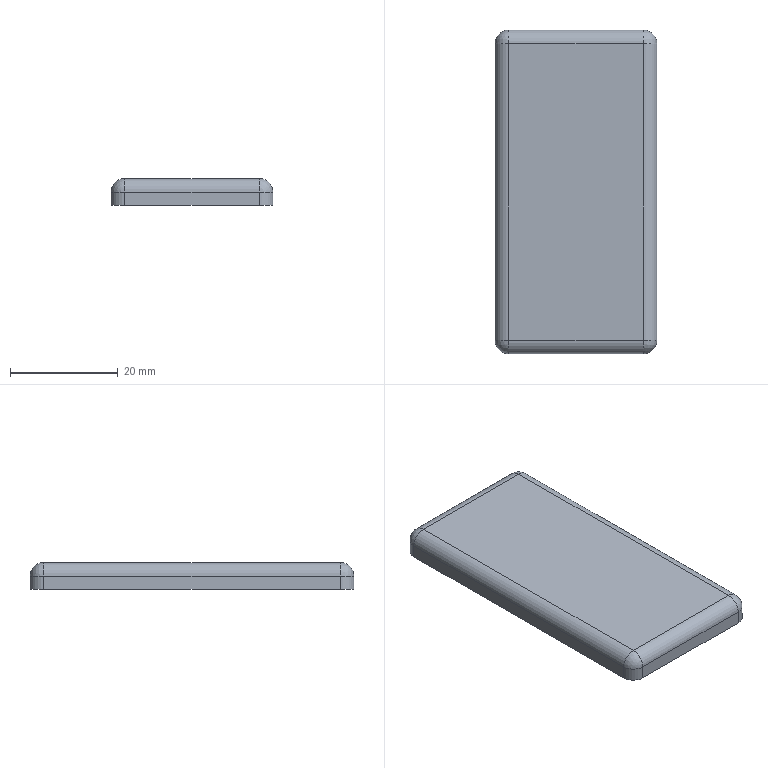Part | STEP file | Aluminium profile end cover plate | 1 solid | 18 faces | box 30 x 60 x 5 mm | volume 8742 mm3 | cylinder 8 | plane 6 | sphere 4 | commonest cylinder face diameters 5 x8
STEP:
#1=CARTESIAN_POINT('',(0.,0.,0.));
#2=DIRECTION('',(0.,0.,1.));
#3=DIRECTION('',(1.,0.,0.));
#4=AXIS2_PLACEMENT_3D('',#1,#2,#3);
#5=CARTESIAN_POINT('',(15.,27.5,2.5));
#6=VERTEX_POINT('',#5);
#7=CARTESIAN_POINT('',(15.,-27.5,2.5));
#8=VERTEX_POINT('',#7);
#9=CARTESIAN_POINT('',(15.,-30.,2.5));
#10=DIRECTION('',(0.,-1.,0.));
#11=VECTOR('',#10,1.);
#12=LINE('',#9,#11);
#13=CARTESIAN_POINT('',(15.,30.,5.));
#14=DIRECTION('',(-1.,0.,0.));
#15=DIRECTION('',(0.,-1.,0.));
#16=AXIS2_PLACEMENT_3D('',#13,#14,#15);
#17=PLANE('',#16);
#18=CARTESIAN_POINT('',(60.,-2.5));
#19=DIRECTION('',(1.,0.));
#20=VECTOR('',#19,1.);
#21=LINE('',#18,#20);
#22=(GEOMETRIC_REPRESENTATION_CONTEXT(2)PARAMETRIC_REPRESENTATION_CONTEXT()REPRESENTATION_CONTEXT('',''));
#23=DEFINITIONAL_REPRESENTATION('',(#21),#22);
#24=PCURVE('',#17,#23);
#25=CARTESIAN_POINT('',(12.5,0.,2.5));
#26=DIRECTION('',(0.,-1.,0.));
#27=DIRECTION('',(1.,0.,0.));
#28=AXIS2_PLACEMENT_3D('',#25,#26,#27);
#29=CYLINDRICAL_SURFACE('',#28,2.5);
#30=CARTESIAN_POINT('',(0.,30.));
#31=DIRECTION('',(0.,1.));
#32=VECTOR('',#31,1.);
#33=LINE('',#30,#32);
#34=(GEOMETRIC_REPRESENTATION_CONTEXT(2)PARAMETRIC_REPRESENTATION_CONTEXT()REPRESENTATION_CONTEXT('',''));
#35=DEFINITIONAL_REPRESENTATION('',(#33),#34);
#36=PCURVE('',#29,#35);
#37=SURFACE_CURVE('',#12,(#24,#36),.PCURVE_S1.);
#38=EDGE_CURVE('',#6,#8,#37,.T.);
#39=ORIENTED_EDGE('',*,*,#38,.T.);
#40=CARTESIAN_POINT('',(15.,-27.5,0.));
#41=VERTEX_POINT('',#40);
#42=CARTESIAN_POINT('',(15.,-27.5,5.));
#43=DIRECTION('',(0.,0.,-1.));
#44=VECTOR('',#43,1.);
#45=LINE('',#42,#44);
#46=CARTESIAN_POINT('',(57.5,0.));
#47=DIRECTION('',(0.,-1.));
#48=VECTOR('',#47,1.);
#49=LINE('',#46,#48);
#50=(GEOMETRIC_REPRESENTATION_CONTEXT(2)PARAMETRIC_REPRESENTATION_CONTEXT()REPRESENTATION_CONTEXT('',''));
#51=DEFINITIONAL_REPRESENTATION('',(#49),#50);
#52=PCURVE('',#17,#51);
#53=CARTESIAN_POINT('',(12.5,-27.5,5.));
#54=DIRECTION('',(0.,0.,-1.));
#55=DIRECTION('',(-1.,0.,0.));
#56=AXIS2_PLACEMENT_3D('',#53,#54,#55);
#57=CYLINDRICAL_SURFACE('',#56,2.5);
#58=CARTESIAN_POINT('',(3.142,0.));
#59=DIRECTION('',(0.,1.));
#60=VECTOR('',#59,1.);
#61=LINE('',#58,#60);
#62=(GEOMETRIC_REPRESENTATION_CONTEXT(2)PARAMETRIC_REPRESENTATION_CONTEXT()REPRESENTATION_CONTEXT('',''));
#63=DEFINITIONAL_REPRESENTATION('',(#61),#62);
#64=PCURVE('',#57,#63);
#65=SURFACE_CURVE('',#45,(#52,#64),.PCURVE_S1.);
#66=EDGE_CURVE('',#8,#41,#65,.T.);
#67=ORIENTED_EDGE('',*,*,#66,.T.);
#68=CARTESIAN_POINT('',(15.,27.5,0.));
#69=VERTEX_POINT('',#68);
#70=CARTESIAN_POINT('',(15.,30.,0.));
#71=DIRECTION('',(0.,1.,0.));
#72=VECTOR('',#71,1.);
#73=LINE('',#70,#72);
#74=CARTESIAN_POINT('',(0.,-5.));
#75=DIRECTION('',(-1.,0.));
#76=VECTOR('',#75,1.);
#77=LINE('',#74,#76);
#78=(GEOMETRIC_REPRESENTATION_CONTEXT(2)PARAMETRIC_REPRESENTATION_CONTEXT()REPRESENTATION_CONTEXT('',''));
#79=DEFINITIONAL_REPRESENTATION('',(#77),#78);
#80=PCURVE('',#17,#79);
#81=CARTESIAN_POINT('',(0.,0.,0.));
#82=DIRECTION('',(0.,0.,1.));
#83=DIRECTION('',(1.,0.,0.));
#84=AXIS2_PLACEMENT_3D('',#81,#82,#83);
#85=PLANE('',#84);
#86=CARTESIAN_POINT('',(15.,30.));
#87=DIRECTION('',(0.,1.));
#88=VECTOR('',#87,1.);
#89=LINE('',#86,#88);
#90=(GEOMETRIC_REPRESENTATION_CONTEXT(2)PARAMETRIC_REPRESENTATION_CONTEXT()REPRESENTATION_CONTEXT('',''));
#91=DEFINITIONAL_REPRESENTATION('',(#89),#90);
#92=PCURVE('',#85,#91);
#93=SURFACE_CURVE('',#73,(#80,#92),.PCURVE_S1.);
#94=EDGE_CURVE('',#41,#69,#93,.T.);
#95=ORIENTED_EDGE('',*,*,#94,.T.);
#96=CARTESIAN_POINT('',(15.,27.5,5.));
#97=DIRECTION('',(0.,0.,1.));
#98=VECTOR('',#97,1.);
#99=LINE('',#96,#98);
#100=CARTESIAN_POINT('',(2.5,0.));
#101=DIRECTION('',(0.,1.));
#102=VECTOR('',#101,1.);
#103=LINE('',#100,#102);
#104=(GEOMETRIC_REPRESENTATION_CONTEXT(2)PARAMETRIC_REPRESENTATION_CONTEXT()REPRESENTATION_CONTEXT('',''));
#105=DEFINITIONAL_REPRESENTATION('',(#103),#104);
#106=PCURVE('',#17,#105);
#107=CARTESIAN_POINT('',(12.5,27.5,5.));
#108=DIRECTION('',(0.,0.,-1.));
#109=DIRECTION('',(-1.,0.,0.));
#110=AXIS2_PLACEMENT_3D('',#107,#108,#109);
#111=CYLINDRICAL_SURFACE('',#110,2.5);
#112=CARTESIAN_POINT('',(3.142,0.));
#113=DIRECTION('',(0.,-1.));
#114=VECTOR('',#113,1.);
#115=LINE('',#112,#114);
#116=(GEOMETRIC_REPRESENTATION_CONTEXT(2)PARAMETRIC_REPRESENTATION_CONTEXT()REPRESENTATION_CONTEXT('',''));
#117=DEFINITIONAL_REPRESENTATION('',(#115),#116);
#118=PCURVE('',#111,#117);
#119=SURFACE_CURVE('',#99,(#106,#118),.PCURVE_S1.);
#120=EDGE_CURVE('',#69,#6,#119,.T.);
#121=ORIENTED_EDGE('',*,*,#120,.T.);
#122=EDGE_LOOP('',(#39,#67,#95,#121));
#123=FACE_BOUND('',#122,.T.);
#124=ADVANCED_FACE('',(#123),#17,.F.);
#125=CARTESIAN_POINT('',(12.5,30.,0.));
#126=VERTEX_POINT('',#125);
#127=CARTESIAN_POINT('',(-12.5,30.,0.));
#128=VERTEX_POINT('',#127);
#129=CARTESIAN_POINT('',(-15.,30.,0.));
#130=DIRECTION('',(-1.,0.,0.));
#131=VECTOR('',#130,1.);
#132=LINE('',#129,#131);
#133=CARTESIAN_POINT('',(-15.,30.,5.));
#134=DIRECTION('',(0.,-1.,0.));
#135=DIRECTION('',(0.,0.,-1.));
#136=AXIS2_PLACEMENT_3D('',#133,#134,#135);
#137=PLANE('',#136);
#138=CARTESIAN_POINT('',(5.,0.));
#139=DIRECTION('',(0.,-1.));
#140=VECTOR('',#139,1.);
#141=LINE('',#138,#140);
#142=(GEOMETRIC_REPRESENTATION_CONTEXT(2)PARAMETRIC_REPRESENTATION_CONTEXT()REPRESENTATION_CONTEXT('',''));
#143=DEFINITIONAL_REPRESENTATION('',(#141),#142);
#144=PCURVE('',#137,#143);
#145=CARTESIAN_POINT('',(-15.,30.));
#146=DIRECTION('',(-1.,0.));
#147=VECTOR('',#146,1.);
#148=LINE('',#145,#147);
#149=(GEOMETRIC_REPRESENTATION_CONTEXT(2)PARAMETRIC_REPRESENTATION_CONTEXT()REPRESENTATION_CONTEXT('',''));
#150=DEFINITIONAL_REPRESENTATION('',(#148),#149);
#151=PCURVE('',#85,#150);
#152=SURFACE_CURVE('',#132,(#144,#151),.PCURVE_S1.);
#153=EDGE_CURVE('',#126,#128,#152,.T.);
#154=ORIENTED_EDGE('',*,*,#153,.T.);
#155=CARTESIAN_POINT('',(-12.5,30.,2.5));
#156=VERTEX_POINT('',#155);
#157=CARTESIAN_POINT('',(-12.5,30.,5.));
#158=DIRECTION('',(0.,0.,1.));
#159=VECTOR('',#158,1.);
#160=LINE('',#157,#159);
#161=CARTESIAN_POINT('',(0.,2.5));
#162=DIRECTION('',(-1.,0.));
#163=VECTOR('',#162,1.);
#164=LINE('',#161,#163);
#165=(GEOMETRIC_REPRESENTATION_CONTEXT(2)PARAMETRIC_REPRESENTATION_CONTEXT()REPRESENTATION_CONTEXT('',''));
#166=DEFINITIONAL_REPRESENTATION('',(#164),#165);
#167=PCURVE('',#137,#166);
#168=CARTESIAN_POINT('',(-12.5,27.5,5.));
#169=DIRECTION('',(0.,0.,-1.));
#170=DIRECTION('',(-1.,0.,0.));
#171=AXIS2_PLACEMENT_3D('',#168,#169,#170);
#172=CYLINDRICAL_SURFACE('',#171,2.5);
#173=CARTESIAN_POINT('',(1.571,0.));
#174=DIRECTION('',(0.,-1.));
#175=VECTOR('',#174,1.);
#176=LINE('',#173,#175);
#177=(GEOMETRIC_REPRESENTATION_CONTEXT(2)PARAMETRIC_REPRESENTATION_CONTEXT()REPRESENTATION_CONTEXT('',''));
#178=DEFINITIONAL_REPRESENTATION('',(#176),#177);
#179=PCURVE('',#172,#178);
#180=SURFACE_CURVE('',#160,(#167,#179),.PCURVE_S1.);
#181=EDGE_CURVE('',#128,#156,#180,.T.);
#182=ORIENTED_EDGE('',*,*,#181,.T.);
#183=CARTESIAN_POINT('',(12.5,30.,2.5));
#184=VERTEX_POINT('',#183);
#185=CARTESIAN_POINT('',(15.,30.,2.5));
#186=DIRECTION('',(1.,0.,0.));
#187=VECTOR('',#186,1.);
#188=LINE('',#185,#187);
#189=CARTESIAN_POINT('',(2.5,30.));
#190=DIRECTION('',(0.,1.));
#191=VECTOR('',#190,1.);
#192=LINE('',#189,#191);
#193=(GEOMETRIC_REPRESENTATION_CONTEXT(2)PARAMETRIC_REPRESENTATION_CONTEXT()REPRESENTATION_CONTEXT('',''));
#194=DEFINITIONAL_REPRESENTATION('',(#192),#193);
#195=PCURVE('',#137,#194);
#196=CARTESIAN_POINT('',(0.,27.5,2.5));
#197=DIRECTION('',(1.,0.,0.));
#198=DIRECTION('',(0.,0.,-1.));
#199=AXIS2_PLACEMENT_3D('',#196,#197,#198);
#200=CYLINDRICAL_SURFACE('',#199,2.5);
#201=CARTESIAN_POINT('',(1.571,15.));
#202=DIRECTION('',(0.,1.));
#203=VECTOR('',#202,1.);
#204=LINE('',#201,#203);
#205=(GEOMETRIC_REPRESENTATION_CONTEXT(2)PARAMETRIC_REPRESENTATION_CONTEXT()REPRESENTATION_CONTEXT('',''));
#206=DEFINITIONAL_REPRESENTATION('',(#204),#205);
#207=PCURVE('',#200,#206);
#208=SURFACE_CURVE('',#188,(#195,#207),.PCURVE_S1.);
#209=EDGE_CURVE('',#156,#184,#208,.T.);
#210=ORIENTED_EDGE('',*,*,#209,.T.);
#211=CARTESIAN_POINT('',(12.5,30.,5.));
#212=DIRECTION('',(0.,0.,-1.));
#213=VECTOR('',#212,1.);
#214=LINE('',#211,#213);
#215=CARTESIAN_POINT('',(0.,27.5));
#216=DIRECTION('',(1.,0.));
#217=VECTOR('',#216,1.);
#218=LINE('',#215,#217);
#219=(GEOMETRIC_REPRESENTATION_CONTEXT(2)PARAMETRIC_REPRESENTATION_CONTEXT()REPRESENTATION_CONTEXT('',''));
#220=DEFINITIONAL_REPRESENTATION('',(#218),#219);
#221=PCURVE('',#137,#220);
#222=CARTESIAN_POINT('',(1.571,0.));
#223=DIRECTION('',(0.,1.));
#224=VECTOR('',#223,1.);
#225=LINE('',#222,#224);
#226=(GEOMETRIC_REPRESENTATION_CONTEXT(2)PARAMETRIC_REPRESENTATION_CONTEXT()REPRESENTATION_CONTEXT('',''));
#227=DEFINITIONAL_REPRESENTATION('',(#225),#226);
#228=PCURVE('',#111,#227);
#229=SURFACE_CURVE('',#214,(#221,#228),.PCURVE_S1.);
#230=EDGE_CURVE('',#184,#126,#229,.T.);
#231=ORIENTED_EDGE('',*,*,#230,.T.);
#232=EDGE_LOOP('',(#154,#182,#210,#231));
#233=FACE_BOUND('',#232,.T.);
#234=ADVANCED_FACE('',(#233),#137,.F.);
#235=CARTESIAN_POINT('',(-15.,27.5,0.));
#236=VERTEX_POINT('',#235);
#237=CARTESIAN_POINT('',(-15.,-27.5,0.));
#238=VERTEX_POINT('',#237);
#239=CARTESIAN_POINT('',(-15.,30.,0.));
#240=DIRECTION('',(0.,-1.,0.));
#241=VECTOR('',#240,1.);
#242=LINE('',#239,#241);
#243=CARTESIAN_POINT('',(-15.,30.,5.));
#244=DIRECTION('',(1.,0.,0.));
#245=DIRECTION('',(0.,1.,0.));
#246=AXIS2_PLACEMENT_3D('',#243,#244,#245);
#247=PLANE('',#246);
#248=CARTESIAN_POINT('',(0.,-5.));
#249=DIRECTION('',(-1.,0.));
#250=VECTOR('',#249,1.);
#251=LINE('',#248,#250);
#252=(GEOMETRIC_REPRESENTATION_CONTEXT(2)PARAMETRIC_REPRESENTATION_CONTEXT()REPRESENTATION_CONTEXT('',''));
#253=DEFINITIONAL_REPRESENTATION('',(#251),#252);
#254=PCURVE('',#247,#253);
#255=CARTESIAN_POINT('',(-15.,30.));
#256=DIRECTION('',(0.,-1.));
#257=VECTOR('',#256,1.);
#258=LINE('',#255,#257);
#259=(GEOMETRIC_REPRESENTATION_CONTEXT(2)PARAMETRIC_REPRESENTATION_CONTEXT()REPRESENTATION_CONTEXT('',''));
#260=DEFINITIONAL_REPRESENTATION('',(#258),#259);
#261=PCURVE('',#85,#260);
#262=SURFACE_CURVE('',#242,(#254,#261),.PCURVE_S1.);
#263=EDGE_CURVE('',#236,#238,#262,.T.);
#264=ORIENTED_EDGE('',*,*,#263,.T.);
#265=CARTESIAN_POINT('',(-15.,-27.5,2.5));
#266=VERTEX_POINT('',#265);
#267=CARTESIAN_POINT('',(-15.,-27.5,5.));
#268=DIRECTION('',(0.,0.,1.));
#269=VECTOR('',#268,1.);
#270=LINE('',#267,#269);
#271=CARTESIAN_POINT('',(-57.5,0.));
#272=DIRECTION('',(0.,1.));
#273=VECTOR('',#272,1.);
#274=LINE('',#271,#273);
#275=(GEOMETRIC_REPRESENTATION_CONTEXT(2)PARAMETRIC_REPRESENTATION_CONTEXT()REPRESENTATION_CONTEXT('',''));
#276=DEFINITIONAL_REPRESENTATION('',(#274),#275);
#277=PCURVE('',#247,#276);
#278=CARTESIAN_POINT('',(-12.5,-27.5,5.));
#279=DIRECTION('',(0.,0.,-1.));
#280=DIRECTION('',(-1.,0.,0.));
#281=AXIS2_PLACEMENT_3D('',#278,#279,#280);
#282=CYLINDRICAL_SURFACE('',#281,2.5);
#283=CARTESIAN_POINT('',(6.283,0.));
#284=DIRECTION('',(0.,-1.));
#285=VECTOR('',#284,1.);
#286=LINE('',#283,#285);
#287=(GEOMETRIC_REPRESENTATION_CONTEXT(2)PARAMETRIC_REPRESENTATION_CONTEXT()REPRESENTATION_CONTEXT('',''));
#288=DEFINITIONAL_REPRESENTATION('',(#286),#287);
#289=PCURVE('',#282,#288);
#290=SURFACE_CURVE('',#270,(#277,#289),.PCURVE_S1.);
#291=EDGE_CURVE('',#238,#266,#290,.T.);
#292=ORIENTED_EDGE('',*,*,#291,.T.);
#293=CARTESIAN_POINT('',(-15.,27.5,2.5));
#294=VERTEX_POINT('',#293);
#295=CARTESIAN_POINT('',(-15.,30.,2.5));
#296=DIRECTION('',(0.,1.,0.));
#297=VECTOR('',#296,1.);
#298=LINE('',#295,#297);
#299=CARTESIAN_POINT('',(0.,-2.5));
#300=DIRECTION('',(1.,0.));
#301=VECTOR('',#300,1.);
#302=LINE('',#299,#301);
#303=(GEOMETRIC_REPRESENTATION_CONTEXT(2)PARAMETRIC_REPRESENTATION_CONTEXT()REPRESENTATION_CONTEXT('',''));
#304=DEFINITIONAL_REPRESENTATION('',(#302),#303);
#305=PCURVE('',#247,#304);
#306=CARTESIAN_POINT('',(-12.5,0.,2.5));
#307=DIRECTION('',(0.,1.,0.));
#308=DIRECTION('',(-1.,0.,0.));
#309=AXIS2_PLACEMENT_3D('',#306,#307,#308);
#310=CYLINDRICAL_SURFACE('',#309,2.5);
#311=CARTESIAN_POINT('',(0.,30.));
#312=DIRECTION('',(0.,1.));
#313=VECTOR('',#312,1.);
#314=LINE('',#311,#313);
#315=(GEOMETRIC_REPRESENTATION_CONTEXT(2)PARAMETRIC_REPRESENTATION_CONTEXT()REPRESENTATION_CONTEXT('',''));
#316=DEFINITIONAL_REPRESENTATION('',(#314),#315);
#317=PCURVE('',#310,#316);
#318=SURFACE_CURVE('',#298,(#305,#317),.PCURVE_S1.);
#319=EDGE_CURVE('',#266,#294,#318,.T.);
#320=ORIENTED_EDGE('',*,*,#319,.T.);
#321=CARTESIAN_POINT('',(-15.,27.5,5.));
#322=DIRECTION('',(0.,0.,-1.));
#323=VECTOR('',#322,1.);
#324=LINE('',#321,#323);
#325=CARTESIAN_POINT('',(-2.5,0.));
#326=DIRECTION('',(0.,-1.));
#327=VECTOR('',#326,1.);
#328=LINE('',#325,#327);
#329=(GEOMETRIC_REPRESENTATION_CONTEXT(2)PARAMETRIC_REPRESENTATION_CONTEXT()REPRESENTATION_CONTEXT('',''));
#330=DEFINITIONAL_REPRESENTATION('',(#328),#329);
#331=PCURVE('',#247,#330);
#332=CARTESIAN_POINT('',(0.,0.));
#333=DIRECTION('',(0.,1.));
#334=VECTOR('',#333,1.);
#335=LINE('',#332,#334);
#336=(GEOMETRIC_REPRESENTATION_CONTEXT(2)PARAMETRIC_REPRESENTATION_CONTEXT()REPRESENTATION_CONTEXT('',''));
#337=DEFINITIONAL_REPRESENTATION('',(#335),#336);
#338=PCURVE('',#172,#337);
#339=SURFACE_CURVE('',#324,(#331,#338),.PCURVE_S1.);
#340=EDGE_CURVE('',#294,#236,#339,.T.);
#341=ORIENTED_EDGE('',*,*,#340,.T.);
#342=EDGE_LOOP('',(#264,#292,#320,#341));
#343=FACE_BOUND('',#342,.T.);
#344=ADVANCED_FACE('',(#343),#247,.F.);
#345=CARTESIAN_POINT('',(-12.5,-30.,0.));
#346=VERTEX_POINT('',#345);
#347=CARTESIAN_POINT('',(12.5,-30.,0.));
#348=VERTEX_POINT('',#347);
#349=CARTESIAN_POINT('',(-15.,-30.,0.));
#350=DIRECTION('',(1.,0.,0.));
#351=VECTOR('',#350,1.);
#352=LINE('',#349,#351);
#353=CARTESIAN_POINT('',(-15.,-30.,5.));
#354=DIRECTION('',(0.,1.,0.));
#355=DIRECTION('',(0.,0.,1.));
#356=AXIS2_PLACEMENT_3D('',#353,#354,#355);
#357=PLANE('',#356);
#358=CARTESIAN_POINT('',(-5.,0.));
#359=DIRECTION('',(0.,1.));
#360=VECTOR('',#359,1.);
#361=LINE('',#358,#360);
#362=(GEOMETRIC_REPRESENTATION_CONTEXT(2)PARAMETRIC_REPRESENTATION_CONTEXT()REPRESENTATION_CONTEXT('',''));
#363=DEFINITIONAL_REPRESENTATION('',(#361),#362);
#364=PCURVE('',#357,#363);
#365=CARTESIAN_POINT('',(-15.,-30.));
#366=DIRECTION('',(1.,0.));
#367=VECTOR('',#366,1.);
#368=LINE('',#365,#367);
#369=(GEOMETRIC_REPRESENTATION_CONTEXT(2)PARAMETRIC_REPRESENTATION_CONTEXT()REPRESENTATION_CONTEXT('',''));
#370=DEFINITIONAL_REPRESENTATION('',(#368),#369);
#371=PCURVE('',#85,#370);
#372=SURFACE_CURVE('',#352,(#364,#371),.PCURVE_S1.);
#373=EDGE_CURVE('',#346,#348,#372,.T.);
#374=ORIENTED_EDGE('',*,*,#373,.T.);
#375=CARTESIAN_POINT('',(12.5,-30.,2.5));
#376=VERTEX_POINT('',#375);
#377=CARTESIAN_POINT('',(12.5,-30.,5.));
#378=DIRECTION('',(0.,0.,1.));
#379=VECTOR('',#378,1.);
#380=LINE('',#377,#379);
#381=CARTESIAN_POINT('',(0.,27.5));
#382=DIRECTION('',(1.,0.));
#383=VECTOR('',#382,1.);
#384=LINE('',#381,#383);
#385=(GEOMETRIC_REPRESENTATION_CONTEXT(2)PARAMETRIC_REPRESENTATION_CONTEXT()REPRESENTATION_CONTEXT('',''));
#386=DEFINITIONAL_REPRESENTATION('',(#384),#385);
#387=PCURVE('',#357,#386);
#388=CARTESIAN_POINT('',(4.712,0.));
#389=DIRECTION('',(0.,-1.));
#390=VECTOR('',#389,1.);
#391=LINE('',#388,#390);
#392=(GEOMETRIC_REPRESENTATION_CONTEXT(2)PARAMETRIC_REPRESENTATION_CONTEXT()REPRESENTATION_CONTEXT('',''));
#393=DEFINITIONAL_REPRESENTATION('',(#391),#392);
#394=PCURVE('',#57,#393);
#395=SURFACE_CURVE('',#380,(#387,#394),.PCURVE_S1.);
#396=EDGE_CURVE('',#348,#376,#395,.T.);
#397=ORIENTED_EDGE('',*,*,#396,.T.);
#398=CARTESIAN_POINT('',(-12.5,-30.,2.5));
#399=VERTEX_POINT('',#398);
#400=CARTESIAN_POINT('',(-15.,-30.,2.5));
#401=DIRECTION('',(-1.,0.,0.));
#402=VECTOR('',#401,1.);
#403=LINE('',#400,#402);
#404=CARTESIAN_POINT('',(-2.5,0.));
#405=DIRECTION('',(0.,-1.));
#406=VECTOR('',#405,1.);
#407=LINE('',#404,#406);
#408=(GEOMETRIC_REPRESENTATION_CONTEXT(2)PARAMETRIC_REPRESENTATION_CONTEXT()REPRESENTATION_CONTEXT('',''));
#409=DEFINITIONAL_REPRESENTATION('',(#407),#408);
#410=PCURVE('',#357,#409);
#411=CARTESIAN_POINT('',(0.,-27.5,2.5));
#412=DIRECTION('',(-1.,0.,0.));
#413=DIRECTION('',(0.,0.,1.));
#414=AXIS2_PLACEMENT_3D('',#411,#412,#413);
#415=CYLINDRICAL_SURFACE('',#414,2.5);
#416=CARTESIAN_POINT('',(4.712,15.));
#417=DIRECTION('',(0.,1.));
#418=VECTOR('',#417,1.);
#419=LINE('',#416,#418);
#420=(GEOMETRIC_REPRESENTATION_CONTEXT(2)PARAMETRIC_REPRESENTATION_CONTEXT()REPRESENTATION_CONTEXT('',''));
#421=DEFINITIONAL_REPRESENTATION('',(#419),#420);
#422=PCURVE('',#415,#421);
#423=SURFACE_CURVE('',#403,(#410,#422),.PCURVE_S1.);
#424=EDGE_CURVE('',#376,#399,#423,.T.);
#425=ORIENTED_EDGE('',*,*,#424,.T.);
#426=CARTESIAN_POINT('',(-12.5,-30.,5.));
#427=DIRECTION('',(0.,0.,-1.));
#428=VECTOR('',#427,1.);
#429=LINE('',#426,#428);
#430=CARTESIAN_POINT('',(0.,2.5));
#431=DIRECTION('',(-1.,0.));
#432=VECTOR('',#431,1.);
#433=LINE('',#430,#432);
#434=(GEOMETRIC_REPRESENTATION_CONTEXT(2)PARAMETRIC_REPRESENTATION_CONTEXT()REPRESENTATION_CONTEXT('',''));
#435=DEFINITIONAL_REPRESENTATION('',(#433),#434);
#436=PCURVE('',#357,#435);
#437=CARTESIAN_POINT('',(4.712,0.));
#438=DIRECTION('',(0.,1.));
#439=VECTOR('',#438,1.);
#440=LINE('',#437,#439);
#441=(GEOMETRIC_REPRESENTATION_CONTEXT(2)PARAMETRIC_REPRESENTATION_CONTEXT()REPRESENTATION_CONTEXT('',''));
#442=DEFINITIONAL_REPRESENTATION('',(#440),#441);
#443=PCURVE('',#282,#442);
#444=SURFACE_CURVE('',#429,(#436,#443),.PCURVE_S1.);
#445=EDGE_CURVE('',#399,#346,#444,.T.);
#446=ORIENTED_EDGE('',*,*,#445,.T.);
#447=EDGE_LOOP('',(#374,#397,#425,#446));
#448=FACE_BOUND('',#447,.T.);
#449=ADVANCED_FACE('',(#448),#357,.F.);
#450=CARTESIAN_POINT('',(-12.5,27.5,5.));
#451=VERTEX_POINT('',#450);
#452=CARTESIAN_POINT('',(-12.5,-27.5,5.));
#453=VERTEX_POINT('',#452);
#454=CARTESIAN_POINT('',(-12.5,-30.,5.));
#455=DIRECTION('',(0.,-1.,0.));
#456=VECTOR('',#455,1.);
#457=LINE('',#454,#456);
#458=CARTESIAN_POINT('',(0.,0.,5.));
#459=DIRECTION('',(0.,0.,1.));
#460=DIRECTION('',(1.,0.,0.));
#461=AXIS2_PLACEMENT_3D('',#458,#459,#460);
#462=PLANE('',#461);
#463=CARTESIAN_POINT('',(-12.5,-30.));
#464=DIRECTION('',(0.,-1.));
#465=VECTOR('',#464,1.);
#466=LINE('',#463,#465);
#467=(GEOMETRIC_REPRESENTATION_CONTEXT(2)PARAMETRIC_REPRESENTATION_CONTEXT()REPRESENTATION_CONTEXT('',''));
#468=DEFINITIONAL_REPRESENTATION('',(#466),#467);
#469=PCURVE('',#462,#468);
#470=CARTESIAN_POINT('',(1.571,-30.));
#471=DIRECTION('',(0.,-1.));
#472=VECTOR('',#471,1.);
#473=LINE('',#470,#472);
#474=(GEOMETRIC_REPRESENTATION_CONTEXT(2)PARAMETRIC_REPRESENTATION_CONTEXT()REPRESENTATION_CONTEXT('',''));
#475=DEFINITIONAL_REPRESENTATION('',(#473),#474);
#476=PCURVE('',#310,#475);
#477=SURFACE_CURVE('',#457,(#469,#476),.PCURVE_S1.);
#478=EDGE_CURVE('',#451,#453,#477,.T.);
#479=ORIENTED_EDGE('',*,*,#478,.T.);
#480=CARTESIAN_POINT('',(12.5,-27.5,5.));
#481=VERTEX_POINT('',#480);
#482=CARTESIAN_POINT('',(15.,-27.5,5.));
#483=DIRECTION('',(1.,0.,0.));
#484=VECTOR('',#483,1.);
#485=LINE('',#482,#484);
#486=CARTESIAN_POINT('',(15.,-27.5));
#487=DIRECTION('',(1.,0.));
#488=VECTOR('',#487,1.);
#489=LINE('',#486,#488);
#490=(GEOMETRIC_REPRESENTATION_CONTEXT(2)PARAMETRIC_REPRESENTATION_CONTEXT()REPRESENTATION_CONTEXT('',''));
#491=DEFINITIONAL_REPRESENTATION('',(#489),#490);
#492=PCURVE('',#462,#491);
#493=CARTESIAN_POINT('',(6.283,-15.));
#494=DIRECTION('',(0.,-1.));
#495=VECTOR('',#494,1.);
#496=LINE('',#493,#495);
#497=(GEOMETRIC_REPRESENTATION_CONTEXT(2)PARAMETRIC_REPRESENTATION_CONTEXT()REPRESENTATION_CONTEXT('',''));
#498=DEFINITIONAL_REPRESENTATION('',(#496),#497);
#499=PCURVE('',#415,#498);
#500=SURFACE_CURVE('',#485,(#492,#499),.PCURVE_S1.);
#501=EDGE_CURVE('',#453,#481,#500,.T.);
#502=ORIENTED_EDGE('',*,*,#501,.T.);
#503=CARTESIAN_POINT('',(12.5,27.5,5.));
#504=VERTEX_POINT('',#503);
#505=CARTESIAN_POINT('',(12.5,30.,5.));
#506=DIRECTION('',(0.,1.,0.));
#507=VECTOR('',#506,1.);
#508=LINE('',#505,#507);
#509=CARTESIAN_POINT('',(12.5,30.));
#510=DIRECTION('',(0.,1.));
#511=VECTOR('',#510,1.);
#512=LINE('',#509,#511);
#513=(GEOMETRIC_REPRESENTATION_CONTEXT(2)PARAMETRIC_REPRESENTATION_CONTEXT()REPRESENTATION_CONTEXT('',''));
#514=DEFINITIONAL_REPRESENTATION('',(#512),#513);
#515=PCURVE('',#462,#514);
#516=CARTESIAN_POINT('',(1.571,-30.));
#517=DIRECTION('',(0.,-1.));
#518=VECTOR('',#517,1.);
#519=LINE('',#516,#518);
#520=(GEOMETRIC_REPRESENTATION_CONTEXT(2)PARAMETRIC_REPRESENTATION_CONTEXT()REPRESENTATION_CONTEXT('',''));
#521=DEFINITIONAL_REPRESENTATION('',(#519),#520);
#522=PCURVE('',#29,#521);
#523=SURFACE_CURVE('',#508,(#515,#522),.PCURVE_S1.);
#524=EDGE_CURVE('',#481,#504,#523,.T.);
#525=ORIENTED_EDGE('',*,*,#524,.T.);
#526=CARTESIAN_POINT('',(-15.,27.5,5.));
#527=DIRECTION('',(-1.,0.,0.));
#528=VECTOR('',#527,1.);
#529=LINE('',#526,#528);
#530=CARTESIAN_POINT('',(-15.,27.5));
#531=DIRECTION('',(-1.,0.));
#532=VECTOR('',#531,1.);
#533=LINE('',#530,#532);
#534=(GEOMETRIC_REPRESENTATION_CONTEXT(2)PARAMETRIC_REPRESENTATION_CONTEXT()REPRESENTATION_CONTEXT('',''));
#535=DEFINITIONAL_REPRESENTATION('',(#533),#534);
#536=PCURVE('',#462,#535);
#537=CARTESIAN_POINT('',(3.142,-15.));
#538=DIRECTION('',(0.,-1.));
#539=VECTOR('',#538,1.);
#540=LINE('',#537,#539);
#541=(GEOMETRIC_REPRESENTATION_CONTEXT(2)PARAMETRIC_REPRESENTATION_CONTEXT()REPRESENTATION_CONTEXT('',''));
#542=DEFINITIONAL_REPRESENTATION('',(#540),#541);
#543=PCURVE('',#200,#542);
#544=SURFACE_CURVE('',#529,(#536,#543),.PCURVE_S1.);
#545=EDGE_CURVE('',#504,#451,#544,.T.);
#546=ORIENTED_EDGE('',*,*,#545,.T.);
#547=EDGE_LOOP('',(#479,#502,#525,#546));
#548=FACE_BOUND('',#547,.T.);
#549=ADVANCED_FACE('',(#548),#462,.T.);
#550=ORIENTED_EDGE('',*,*,#94,.F.);
#551=CARTESIAN_POINT('',(12.5,-27.5,0.));
#552=DIRECTION('',(0.,0.,-1.));
#553=DIRECTION('',(1.,0.,0.));
#554=AXIS2_PLACEMENT_3D('',#551,#552,#553);
#555=CIRCLE('',#554,2.5);
#556=CARTESIAN_POINT('',(15.,-27.5));
#557=CARTESIAN_POINT('',(15.,-31.83));
#558=CARTESIAN_POINT('',(11.25,-29.665));
#559=CARTESIAN_POINT('',(7.5,-27.5));
#560=CARTESIAN_POINT('',(11.25,-25.335));
#561=CARTESIAN_POINT('',(15.,-23.17));
#562=CARTESIAN_POINT('',(15.,-27.5));
#563=(BOUNDED_CURVE()B_SPLINE_CURVE(2,(#556,#557,#558,#559,#560,#561,#562),.UNSPECIFIED.,.T.,.F.)B_SPLINE_CURVE_WITH_KNOTS((1,2,2,2,2,1),(-2.094,0.,2.094,4.189,6.283,8.378),.UNSPECIFIED.)CURVE()GEOMETRIC_REPRESENTATION_ITEM()RATIONAL_B_SPLINE_CURVE((1.,0.5,1.,0.5,1.,0.5,1.))REPRESENTATION_ITEM(''));
#564=(GEOMETRIC_REPRESENTATION_CONTEXT(2)PARAMETRIC_REPRESENTATION_CONTEXT()REPRESENTATION_CONTEXT('',''));
#565=DEFINITIONAL_REPRESENTATION('',(#563),#564);
#566=PCURVE('',#85,#565);
#567=CARTESIAN_POINT('',(3.142,5.));
#568=DIRECTION('',(1.,0.));
#569=VECTOR('',#568,1.);
#570=LINE('',#567,#569);
#571=(GEOMETRIC_REPRESENTATION_CONTEXT(2)PARAMETRIC_REPRESENTATION_CONTEXT()REPRESENTATION_CONTEXT('',''));
#572=DEFINITIONAL_REPRESENTATION('',(#570),#571);
#573=PCURVE('',#57,#572);
#574=SURFACE_CURVE('',#555,(#566,#573),.PCURVE_S1.);
#575=EDGE_CURVE('',#41,#348,#574,.T.);
#576=ORIENTED_EDGE('',*,*,#575,.T.);
#577=ORIENTED_EDGE('',*,*,#373,.F.);
#578=CARTESIAN_POINT('',(-12.5,-27.5,0.));
#579=DIRECTION('',(0.,0.,-1.));
#580=DIRECTION('',(1.,0.,0.));
#581=AXIS2_PLACEMENT_3D('',#578,#579,#580);
#582=CIRCLE('',#581,2.5);
#583=CARTESIAN_POINT('',(-10.,-27.5));
#584=CARTESIAN_POINT('',(-10.,-31.83));
#585=CARTESIAN_POINT('',(-13.75,-29.665));
#586=CARTESIAN_POINT('',(-17.5,-27.5));
#587=CARTESIAN_POINT('',(-13.75,-25.335));
#588=CARTESIAN_POINT('',(-10.,-23.17));
#589=CARTESIAN_POINT('',(-10.,-27.5));
#590=(BOUNDED_CURVE()B_SPLINE_CURVE(2,(#583,#584,#585,#586,#587,#588,#589),.UNSPECIFIED.,.T.,.F.)B_SPLINE_CURVE_WITH_KNOTS((1,2,2,2,2,1),(-2.094,0.,2.094,4.189,6.283,8.378),.UNSPECIFIED.)CURVE()GEOMETRIC_REPRESENTATION_ITEM()RATIONAL_B_SPLINE_CURVE((1.,0.5,1.,0.5,1.,0.5,1.))REPRESENTATION_ITEM(''));
#591=(GEOMETRIC_REPRESENTATION_CONTEXT(2)PARAMETRIC_REPRESENTATION_CONTEXT()REPRESENTATION_CONTEXT('',''));
#592=DEFINITIONAL_REPRESENTATION('',(#590),#591);
#593=PCURVE('',#85,#592);
#594=CARTESIAN_POINT('',(3.142,5.));
#595=DIRECTION('',(1.,0.));
#596=VECTOR('',#595,1.);
#597=LINE('',#594,#596);
#598=(GEOMETRIC_REPRESENTATION_CONTEXT(2)PARAMETRIC_REPRESENTATION_CONTEXT()REPRESENTATION_CONTEXT('',''));
#599=DEFINITIONAL_REPRESENTATION('',(#597),#598);
#600=PCURVE('',#282,#599);
#601=SURFACE_CURVE('',#582,(#593,#600),.PCURVE_S1.);
#602=EDGE_CURVE('',#346,#238,#601,.T.);
#603=ORIENTED_EDGE('',*,*,#602,.T.);
#604=ORIENTED_EDGE('',*,*,#263,.F.);
#605=CARTESIAN_POINT('',(-12.5,27.5,0.));
#606=DIRECTION('',(0.,0.,-1.));
#607=DIRECTION('',(1.,0.,0.));
#608=AXIS2_PLACEMENT_3D('',#605,#606,#607);
#609=CIRCLE('',#608,2.5);
#610=CARTESIAN_POINT('',(-10.,27.5));
#611=CARTESIAN_POINT('',(-10.,23.17));
#612=CARTESIAN_POINT('',(-13.75,25.335));
#613=CARTESIAN_POINT('',(-17.5,27.5));
#614=CARTESIAN_POINT('',(-13.75,29.665));
#615=CARTESIAN_POINT('',(-10.,31.83));
#616=CARTESIAN_POINT('',(-10.,27.5));
#617=(BOUNDED_CURVE()B_SPLINE_CURVE(2,(#610,#611,#612,#613,#614,#615,#616),.UNSPECIFIED.,.T.,.F.)B_SPLINE_CURVE_WITH_KNOTS((1,2,2,2,2,1),(-2.094,0.,2.094,4.189,6.283,8.378),.UNSPECIFIED.)CURVE()GEOMETRIC_REPRESENTATION_ITEM()RATIONAL_B_SPLINE_CURVE((1.,0.5,1.,0.5,1.,0.5,1.))REPRESENTATION_ITEM(''));
#618=(GEOMETRIC_REPRESENTATION_CONTEXT(2)PARAMETRIC_REPRESENTATION_CONTEXT()REPRESENTATION_CONTEXT('',''));
#619=DEFINITIONAL_REPRESENTATION('',(#617),#618);
#620=PCURVE('',#85,#619);
#621=CARTESIAN_POINT('',(-3.142,5.));
#622=DIRECTION('',(1.,0.));
#623=VECTOR('',#622,1.);
#624=LINE('',#621,#623);
#625=(GEOMETRIC_REPRESENTATION_CONTEXT(2)PARAMETRIC_REPRESENTATION_CONTEXT()REPRESENTATION_CONTEXT('',''));
#626=DEFINITIONAL_REPRESENTATION('',(#624),#625);
#627=PCURVE('',#172,#626);
#628=SURFACE_CURVE('',#609,(#620,#627),.PCURVE_S1.);
#629=EDGE_CURVE('',#236,#128,#628,.T.);
#630=ORIENTED_EDGE('',*,*,#629,.T.);
#631=ORIENTED_EDGE('',*,*,#153,.F.);
#632=CARTESIAN_POINT('',(12.5,27.5,0.));
#633=DIRECTION('',(0.,0.,-1.));
#634=DIRECTION('',(1.,0.,0.));
#635=AXIS2_PLACEMENT_3D('',#632,#633,#634);
#636=CIRCLE('',#635,2.5);
#637=CARTESIAN_POINT('',(15.,27.5));
#638=CARTESIAN_POINT('',(15.,23.17));
#639=CARTESIAN_POINT('',(11.25,25.335));
#640=CARTESIAN_POINT('',(7.5,27.5));
#641=CARTESIAN_POINT('',(11.25,29.665));
#642=CARTESIAN_POINT('',(15.,31.83));
#643=CARTESIAN_POINT('',(15.,27.5));
#644=(BOUNDED_CURVE()B_SPLINE_CURVE(2,(#637,#638,#639,#640,#641,#642,#643),.UNSPECIFIED.,.T.,.F.)B_SPLINE_CURVE_WITH_KNOTS((1,2,2,2,2,1),(-2.094,0.,2.094,4.189,6.283,8.378),.UNSPECIFIED.)CURVE()GEOMETRIC_REPRESENTATION_ITEM()RATIONAL_B_SPLINE_CURVE((1.,0.5,1.,0.5,1.,0.5,1.))REPRESENTATION_ITEM(''));
#645=(GEOMETRIC_REPRESENTATION_CONTEXT(2)PARAMETRIC_REPRESENTATION_CONTEXT()REPRESENTATION_CONTEXT('',''));
#646=DEFINITIONAL_REPRESENTATION('',(#644),#645);
#647=PCURVE('',#85,#646);
#648=CARTESIAN_POINT('',(-3.142,5.));
#649=DIRECTION('',(1.,0.));
#650=VECTOR('',#649,1.);
#651=LINE('',#648,#650);
#652=(GEOMETRIC_REPRESENTATION_CONTEXT(2)PARAMETRIC_REPRESENTATION_CONTEXT()REPRESENTATION_CONTEXT('',''));
#653=DEFINITIONAL_REPRESENTATION('',(#651),#652);
#654=PCURVE('',#111,#653);
#655=SURFACE_CURVE('',#636,(#647,#654),.PCURVE_S1.);
#656=EDGE_CURVE('',#126,#69,#655,.T.);
#657=ORIENTED_EDGE('',*,*,#656,.T.);
#658=EDGE_LOOP('',(#550,#576,#577,#603,#604,#630,#631,#657));
#659=FACE_BOUND('',#658,.T.);
#660=ADVANCED_FACE('',(#659),#85,.F.);
#661=ORIENTED_EDGE('',*,*,#629,.F.);
#662=ORIENTED_EDGE('',*,*,#340,.F.);
#663=CARTESIAN_POINT('',(-12.5,27.5,2.5));
#664=DIRECTION('',(0.,0.,1.));
#665=DIRECTION('',(1.,0.,0.));
#666=AXIS2_PLACEMENT_3D('',#663,#664,#665);
#667=CIRCLE('',#666,2.5);
#668=CARTESIAN_POINT('',(3.142,2.5));
#669=DIRECTION('',(-1.,0.));
#670=VECTOR('',#669,1.);
#671=LINE('',#668,#670);
#672=(GEOMETRIC_REPRESENTATION_CONTEXT(2)PARAMETRIC_REPRESENTATION_CONTEXT()REPRESENTATION_CONTEXT('',''));
#673=DEFINITIONAL_REPRESENTATION('',(#671),#672);
#674=PCURVE('',#172,#673);
#675=CARTESIAN_POINT('',(-12.5,27.5,2.5));
#676=DIRECTION('',(0.,1.,0.));
#677=DIRECTION('',(1.,0.,0.));
#678=AXIS2_PLACEMENT_3D('',#675,#676,#677);
#679=SPHERICAL_SURFACE('',#678,2.5);
#680=CARTESIAN_POINT('',(3.142,1.571));
#681=CARTESIAN_POINT('',(3.142,1.547));
#682=CARTESIAN_POINT('',(3.142,1.499));
#683=CARTESIAN_POINT('',(3.142,1.428));
#684=CARTESIAN_POINT('',(3.142,1.357));
#685=CARTESIAN_POINT('',(3.142,1.285));
#686=CARTESIAN_POINT('',(3.142,1.214));
#687=CARTESIAN_POINT('',(3.142,1.142));
#688=CARTESIAN_POINT('',(3.142,1.071));
#689=CARTESIAN_POINT('',(3.142,0.9996));
#690=CARTESIAN_POINT('',(3.142,0.9282));
#691=CARTESIAN_POINT('',(3.142,0.8568));
#692=CARTESIAN_POINT('',(3.142,0.7854));
#693=CARTESIAN_POINT('',(3.142,0.714));
#694=CARTESIAN_POINT('',(3.142,0.6426));
#695=CARTESIAN_POINT('',(3.142,0.5712));
#696=CARTESIAN_POINT('',(3.142,0.4998));
#697=CARTESIAN_POINT('',(3.142,0.4284));
#698=CARTESIAN_POINT('',(3.142,0.357));
#699=CARTESIAN_POINT('',(3.142,0.2856));
#700=CARTESIAN_POINT('',(3.142,0.2142));
#701=CARTESIAN_POINT('',(3.142,0.1428));
#702=CARTESIAN_POINT('',(3.142,0.0714));
#703=CARTESIAN_POINT('',(3.142,0.0238));
#704=CARTESIAN_POINT('',(3.142,0.));
#705=B_SPLINE_CURVE_WITH_KNOTS('',3,(#680,#681,#682,#683,#684,#685,#686,#687,#688,#689,#690,#691,#692,#693,#694,#695,#696,#697,#698,#699,#700,#701,#702,#703,#704),.UNSPECIFIED.,.F.,.F.,(4,1,1,1,1,1,1,1,1,1,1,1,1,1,1,1,1,1,1,1,1,1,4),(1.571,1.642,1.714,1.785,1.856,1.928,1.999,2.071,2.142,2.213,2.285,2.356,2.428,2.499,2.57,2.642,2.713,2.785,2.856,2.927,2.999,3.07,3.142),.QUASI_UNIFORM_KNOTS.);
#706=(GEOMETRIC_REPRESENTATION_CONTEXT(2)PARAMETRIC_REPRESENTATION_CONTEXT()REPRESENTATION_CONTEXT('',''));
#707=DEFINITIONAL_REPRESENTATION('',(#705),#706);
#708=PCURVE('',#679,#707);
#709=SURFACE_CURVE('',#667,(#674,#708),.PCURVE_S1.);
#710=EDGE_CURVE('',#156,#294,#709,.T.);
#711=ORIENTED_EDGE('',*,*,#710,.F.);
#712=ORIENTED_EDGE('',*,*,#181,.F.);
#713=EDGE_LOOP('',(#661,#662,#711,#712));
#714=FACE_BOUND('',#713,.T.);
#715=ADVANCED_FACE('',(#714),#172,.T.);
#716=CARTESIAN_POINT('',(12.5,27.5,2.5));
#717=DIRECTION('',(1.,0.,0.));
#718=DIRECTION('',(0.,0.,-1.));
#719=AXIS2_PLACEMENT_3D('',#716,#717,#718);
#720=CIRCLE('',#719,2.5);
#721=CARTESIAN_POINT('',(0.,12.5));
#722=DIRECTION('',(1.,0.));
#723=VECTOR('',#722,1.);
#724=LINE('',#721,#723);
#725=(GEOMETRIC_REPRESENTATION_CONTEXT(2)PARAMETRIC_REPRESENTATION_CONTEXT()REPRESENTATION_CONTEXT('',''));
#726=DEFINITIONAL_REPRESENTATION('',(#724),#725);
#727=PCURVE('',#200,#726);
#728=CARTESIAN_POINT('',(12.5,27.5,2.5));
#729=DIRECTION('',(0.,1.,0.));
#730=DIRECTION('',(1.,0.,0.));
#731=AXIS2_PLACEMENT_3D('',#728,#729,#730);
#732=SPHERICAL_SURFACE('',#731,2.5);
#733=CARTESIAN_POINT('',(4.712,1.571));
#734=CARTESIAN_POINT('',(4.712,1.547));
#735=CARTESIAN_POINT('',(4.712,1.499));
#736=CARTESIAN_POINT('',(4.712,1.428));
#737=CARTESIAN_POINT('',(4.712,1.357));
#738=CARTESIAN_POINT('',(4.712,1.285));
#739=CARTESIAN_POINT('',(4.712,1.214));
#740=CARTESIAN_POINT('',(4.712,1.142));
#741=CARTESIAN_POINT('',(4.712,1.071));
#742=CARTESIAN_POINT('',(4.712,0.9996));
#743=CARTESIAN_POINT('',(4.712,0.9282));
#744=CARTESIAN_POINT('',(4.712,0.8568));
#745=CARTESIAN_POINT('',(4.712,0.7854));
#746=CARTESIAN_POINT('',(4.712,0.714));
#747=CARTESIAN_POINT('',(4.712,0.6426));
#748=CARTESIAN_POINT('',(4.712,0.5712));
#749=CARTESIAN_POINT('',(4.712,0.4998));
#750=CARTESIAN_POINT('',(4.712,0.4284));
#751=CARTESIAN_POINT('',(4.712,0.357));
#752=CARTESIAN_POINT('',(4.712,0.2856));
#753=CARTESIAN_POINT('',(4.712,0.2142));
#754=CARTESIAN_POINT('',(4.712,0.1428));
#755=CARTESIAN_POINT('',(4.712,0.0714));
#756=CARTESIAN_POINT('',(4.712,0.0238));
#757=CARTESIAN_POINT('',(4.712,0.));
#758=B_SPLINE_CURVE_WITH_KNOTS('',3,(#733,#734,#735,#736,#737,#738,#739,#740,#741,#742,#743,#744,#745,#746,#747,#748,#749,#750,#751,#752,#753,#754,#755,#756,#757),.UNSPECIFIED.,.F.,.F.,(4,1,1,1,1,1,1,1,1,1,1,1,1,1,1,1,1,1,1,1,1,1,4),(1.571,1.642,1.714,1.785,1.856,1.928,1.999,2.071,2.142,2.213,2.285,2.356,2.428,2.499,2.57,2.642,2.713,2.785,2.856,2.927,2.999,3.07,3.142),.QUASI_UNIFORM_KNOTS.);
#759=(GEOMETRIC_REPRESENTATION_CONTEXT(2)PARAMETRIC_REPRESENTATION_CONTEXT()REPRESENTATION_CONTEXT('',''));
#760=DEFINITIONAL_REPRESENTATION('',(#758),#759);
#761=PCURVE('',#732,#760);
#762=SURFACE_CURVE('',#720,(#727,#761),.PCURVE_S1.);
#763=EDGE_CURVE('',#184,#504,#762,.T.);
#764=ORIENTED_EDGE('',*,*,#763,.F.);
#765=ORIENTED_EDGE('',*,*,#209,.F.);
#766=CARTESIAN_POINT('',(-12.5,27.5,2.5));
#767=DIRECTION('',(-1.,0.,0.));
#768=DIRECTION('',(0.,0.,1.));
#769=AXIS2_PLACEMENT_3D('',#766,#767,#768);
#770=CIRCLE('',#769,2.5);
#771=CARTESIAN_POINT('',(3.142,-12.5));
#772=DIRECTION('',(-1.,0.));
#773=VECTOR('',#772,1.);
#774=LINE('',#771,#773);
#775=(GEOMETRIC_REPRESENTATION_CONTEXT(2)PARAMETRIC_REPRESENTATION_CONTEXT()REPRESENTATION_CONTEXT('',''));
#776=DEFINITIONAL_REPRESENTATION('',(#774),#775);
#777=PCURVE('',#200,#776);
#778=CARTESIAN_POINT('',(4.712,0.));
#779=CARTESIAN_POINT('',(4.712,0.0238));
#780=CARTESIAN_POINT('',(4.712,0.0714));
#781=CARTESIAN_POINT('',(4.712,0.1428));
#782=CARTESIAN_POINT('',(4.712,0.2142));
#783=CARTESIAN_POINT('',(4.712,0.2856));
#784=CARTESIAN_POINT('',(4.712,0.357));
#785=CARTESIAN_POINT('',(4.712,0.4284));
#786=CARTESIAN_POINT('',(4.712,0.4998));
#787=CARTESIAN_POINT('',(4.712,0.5712));
#788=CARTESIAN_POINT('',(4.712,0.6426));
#789=CARTESIAN_POINT('',(4.712,0.714));
#790=CARTESIAN_POINT('',(4.712,0.7854));
#791=CARTESIAN_POINT('',(4.712,0.8568));
#792=CARTESIAN_POINT('',(4.712,0.9282));
#793=CARTESIAN_POINT('',(4.712,0.9996));
#794=CARTESIAN_POINT('',(4.712,1.071));
#795=CARTESIAN_POINT('',(4.712,1.142));
#796=CARTESIAN_POINT('',(4.712,1.214));
#797=CARTESIAN_POINT('',(4.712,1.285));
#798=CARTESIAN_POINT('',(4.712,1.357));
#799=CARTESIAN_POINT('',(4.712,1.428));
#800=CARTESIAN_POINT('',(4.712,1.499));
#801=CARTESIAN_POINT('',(4.712,1.547));
#802=CARTESIAN_POINT('',(4.712,1.571));
#803=B_SPLINE_CURVE_WITH_KNOTS('',3,(#778,#779,#780,#781,#782,#783,#784,#785,#786,#787,#788,#789,#790,#791,#792,#793,#794,#795,#796,#797,#798,#799,#800,#801,#802),.UNSPECIFIED.,.F.,.F.,(4,1,1,1,1,1,1,1,1,1,1,1,1,1,1,1,1,1,1,1,1,1,4),(0.,0.0714,0.1428,0.2142,0.2856,0.357,0.4284,0.4998,0.5712,0.6426,0.714,0.7854,0.8568,0.9282,0.9996,1.071,1.142,1.214,1.285,1.357,1.428,1.499,1.571),.QUASI_UNIFORM_KNOTS.);
#804=(GEOMETRIC_REPRESENTATION_CONTEXT(2)PARAMETRIC_REPRESENTATION_CONTEXT()REPRESENTATION_CONTEXT('',''));
#805=DEFINITIONAL_REPRESENTATION('',(#803),#804);
#806=PCURVE('',#679,#805);
#807=SURFACE_CURVE('',#770,(#777,#806),.PCURVE_S1.);
#808=EDGE_CURVE('',#451,#156,#807,.T.);
#809=ORIENTED_EDGE('',*,*,#808,.F.);
#810=ORIENTED_EDGE('',*,*,#545,.F.);
#811=EDGE_LOOP('',(#764,#765,#809,#810));
#812=FACE_BOUND('',#811,.T.);
#813=ADVANCED_FACE('',(#812),#200,.T.);
#814=ORIENTED_EDGE('',*,*,#656,.F.);
#815=ORIENTED_EDGE('',*,*,#230,.F.);
#816=CARTESIAN_POINT('',(12.5,27.5,2.5));
#817=DIRECTION('',(0.,0.,1.));
#818=DIRECTION('',(1.,0.,0.));
#819=AXIS2_PLACEMENT_3D('',#816,#817,#818);
#820=CIRCLE('',#819,2.5);
#821=CARTESIAN_POINT('',(3.142,2.5));
#822=DIRECTION('',(-1.,0.));
#823=VECTOR('',#822,1.);
#824=LINE('',#821,#823);
#825=(GEOMETRIC_REPRESENTATION_CONTEXT(2)PARAMETRIC_REPRESENTATION_CONTEXT()REPRESENTATION_CONTEXT('',''));
#826=DEFINITIONAL_REPRESENTATION('',(#824),#825);
#827=PCURVE('',#111,#826);
#828=CARTESIAN_POINT('',(6.283,0.));
#829=CARTESIAN_POINT('',(6.283,0.0238));
#830=CARTESIAN_POINT('',(6.283,0.0714));
#831=CARTESIAN_POINT('',(6.283,0.1428));
#832=CARTESIAN_POINT('',(6.283,0.2142));
#833=CARTESIAN_POINT('',(6.283,0.2856));
#834=CARTESIAN_POINT('',(6.283,0.357));
#835=CARTESIAN_POINT('',(6.283,0.4284));
#836=CARTESIAN_POINT('',(6.283,0.4998));
#837=CARTESIAN_POINT('',(6.283,0.5712));
#838=CARTESIAN_POINT('',(6.283,0.6426));
#839=CARTESIAN_POINT('',(6.283,0.714));
#840=CARTESIAN_POINT('',(6.283,0.7854));
#841=CARTESIAN_POINT('',(6.283,0.8568));
#842=CARTESIAN_POINT('',(6.283,0.9282));
#843=CARTESIAN_POINT('',(6.283,0.9996));
#844=CARTESIAN_POINT('',(6.283,1.071));
#845=CARTESIAN_POINT('',(6.283,1.142));
#846=CARTESIAN_POINT('',(6.283,1.214));
#847=CARTESIAN_POINT('',(6.283,1.285));
#848=CARTESIAN_POINT('',(6.283,1.357));
#849=CARTESIAN_POINT('',(6.283,1.428));
#850=CARTESIAN_POINT('',(6.283,1.499));
#851=CARTESIAN_POINT('',(6.283,1.547));
#852=CARTESIAN_POINT('',(6.283,1.571));
#853=B_SPLINE_CURVE_WITH_KNOTS('',3,(#828,#829,#830,#831,#832,#833,#834,#835,#836,#837,#838,#839,#840,#841,#842,#843,#844,#845,#846,#847,#848,#849,#850,#851,#852),.UNSPECIFIED.,.F.,.F.,(4,1,1,1,1,1,1,1,1,1,1,1,1,1,1,1,1,1,1,1,1,1,4),(0.,0.0714,0.1428,0.2142,0.2856,0.357,0.4284,0.4998,0.5712,0.6426,0.714,0.7854,0.8568,0.9282,0.9996,1.071,1.142,1.214,1.285,1.357,1.428,1.499,1.571),.QUASI_UNIFORM_KNOTS.);
#854=(GEOMETRIC_REPRESENTATION_CONTEXT(2)PARAMETRIC_REPRESENTATION_CONTEXT()REPRESENTATION_CONTEXT('',''));
#855=DEFINITIONAL_REPRESENTATION('',(#853),#854);
#856=PCURVE('',#732,#855);
#857=SURFACE_CURVE('',#820,(#827,#856),.PCURVE_S1.);
#858=EDGE_CURVE('',#6,#184,#857,.T.);
#859=ORIENTED_EDGE('',*,*,#858,.F.);
#860=ORIENTED_EDGE('',*,*,#120,.F.);
#861=EDGE_LOOP('',(#814,#815,#859,#860));
#862=FACE_BOUND('',#861,.T.);
#863=ADVANCED_FACE('',(#862),#111,.T.);
#864=ORIENTED_EDGE('',*,*,#808,.T.);
#865=ORIENTED_EDGE('',*,*,#710,.T.);
#866=CARTESIAN_POINT('',(-12.5,27.5,2.5));
#867=DIRECTION('',(0.,-1.,0.));
#868=DIRECTION('',(0.,0.,1.));
#869=AXIS2_PLACEMENT_3D('',#866,#867,#868);
#870=CIRCLE('',#869,2.5);
#871=CARTESIAN_POINT('',(4.712,0.));
#872=DIRECTION('',(-1.,0.));
#873=VECTOR('',#872,1.);
#874=LINE('',#871,#873);
#875=(GEOMETRIC_REPRESENTATION_CONTEXT(2)PARAMETRIC_REPRESENTATION_CONTEXT()REPRESENTATION_CONTEXT('',''));
#876=DEFINITIONAL_REPRESENTATION('',(#874),#875);
#877=PCURVE('',#679,#876);
#878=CARTESIAN_POINT('',(1.571,27.5));
#879=DIRECTION('',(-1.,0.));
#880=VECTOR('',#879,1.);
#881=LINE('',#878,#880);
#882=(GEOMETRIC_REPRESENTATION_CONTEXT(2)PARAMETRIC_REPRESENTATION_CONTEXT()REPRESENTATION_CONTEXT('',''));
#883=DEFINITIONAL_REPRESENTATION('',(#881),#882);
#884=PCURVE('',#310,#883);
#885=SURFACE_CURVE('',#870,(#877,#884),.PCURVE_S1.);
#886=EDGE_CURVE('',#451,#294,#885,.T.);
#887=ORIENTED_EDGE('',*,*,#886,.F.);
#888=EDGE_LOOP('',(#864,#865,#887));
#889=FACE_BOUND('',#888,.T.);
#890=ADVANCED_FACE('',(#889),#679,.T.);
#891=ORIENTED_EDGE('',*,*,#858,.T.);
#892=ORIENTED_EDGE('',*,*,#763,.T.);
#893=CARTESIAN_POINT('',(12.5,27.5,2.5));
#894=DIRECTION('',(0.,-1.,0.));
#895=DIRECTION('',(0.,0.,1.));
#896=AXIS2_PLACEMENT_3D('',#893,#894,#895);
#897=CIRCLE('',#896,2.5);
#898=CARTESIAN_POINT('',(6.283,0.));
#899=CARTESIAN_POINT('',(6.259,0.));
#900=CARTESIAN_POINT('',(6.212,0.));
#901=CARTESIAN_POINT('',(6.14,0.));
#902=CARTESIAN_POINT('',(6.069,0.));
#903=CARTESIAN_POINT('',(5.998,0.));
#904=CARTESIAN_POINT('',(5.926,0.));
#905=CARTESIAN_POINT('',(5.855,0.));
#906=CARTESIAN_POINT('',(5.783,0.));
#907=CARTESIAN_POINT('',(5.712,0.));
#908=CARTESIAN_POINT('',(5.641,0.));
#909=CARTESIAN_POINT('',(5.569,0.));
#910=CARTESIAN_POINT('',(5.498,0.));
#911=CARTESIAN_POINT('',(5.426,0.));
#912=CARTESIAN_POINT('',(5.355,0.));
#913=CARTESIAN_POINT('',(5.284,0.));
#914=CARTESIAN_POINT('',(5.212,0.));
#915=CARTESIAN_POINT('',(5.141,0.));
#916=CARTESIAN_POINT('',(5.069,0.));
#917=CARTESIAN_POINT('',(4.998,0.));
#918=CARTESIAN_POINT('',(4.927,0.));
#919=CARTESIAN_POINT('',(4.855,0.));
#920=CARTESIAN_POINT('',(4.784,0.));
#921=CARTESIAN_POINT('',(4.736,0.));
#922=CARTESIAN_POINT('',(4.712,0.));
#923=B_SPLINE_CURVE_WITH_KNOTS('',3,(#898,#899,#900,#901,#902,#903,#904,#905,#906,#907,#908,#909,#910,#911,#912,#913,#914,#915,#916,#917,#918,#919,#920,#921,#922),.UNSPECIFIED.,.F.,.F.,(4,1,1,1,1,1,1,1,1,1,1,1,1,1,1,1,1,1,1,1,1,1,4),(4.712,4.784,4.855,4.927,4.998,5.069,5.141,5.212,5.284,5.355,5.426,5.498,5.569,5.641,5.712,5.783,5.855,5.926,5.998,6.069,6.14,6.212,6.283),.QUASI_UNIFORM_KNOTS.);
#924=(GEOMETRIC_REPRESENTATION_CONTEXT(2)PARAMETRIC_REPRESENTATION_CONTEXT()REPRESENTATION_CONTEXT('',''));
#925=DEFINITIONAL_REPRESENTATION('',(#923),#924);
#926=PCURVE('',#732,#925);
#927=CARTESIAN_POINT('',(-4.712,-27.5));
#928=DIRECTION('',(1.,0.));
#929=VECTOR('',#928,1.);
#930=LINE('',#927,#929);
#931=(GEOMETRIC_REPRESENTATION_CONTEXT(2)PARAMETRIC_REPRESENTATION_CONTEXT()REPRESENTATION_CONTEXT('',''));
#932=DEFINITIONAL_REPRESENTATION('',(#930),#931);
#933=PCURVE('',#29,#932);
#934=SURFACE_CURVE('',#897,(#926,#933),.PCURVE_S1.);
#935=EDGE_CURVE('',#6,#504,#934,.T.);
#936=ORIENTED_EDGE('',*,*,#935,.F.);
#937=EDGE_LOOP('',(#891,#892,#936));
#938=FACE_BOUND('',#937,.T.);
#939=ADVANCED_FACE('',(#938),#732,.T.);
#940=ORIENTED_EDGE('',*,*,#602,.F.);
#941=ORIENTED_EDGE('',*,*,#445,.F.);
#942=CARTESIAN_POINT('',(-12.5,-27.5,2.5));
#943=DIRECTION('',(0.,0.,1.));
#944=DIRECTION('',(1.,0.,0.));
#945=AXIS2_PLACEMENT_3D('',#942,#943,#944);
#946=CIRCLE('',#945,2.5);
#947=CARTESIAN_POINT('',(9.425,2.5));
#948=DIRECTION('',(-1.,0.));
#949=VECTOR('',#948,1.);
#950=LINE('',#947,#949);
#951=(GEOMETRIC_REPRESENTATION_CONTEXT(2)PARAMETRIC_REPRESENTATION_CONTEXT()REPRESENTATION_CONTEXT('',''));
#952=DEFINITIONAL_REPRESENTATION('',(#950),#951);
#953=PCURVE('',#282,#952);
#954=CARTESIAN_POINT('',(-12.5,-27.5,2.5));
#955=DIRECTION('',(0.,1.,0.));
#956=DIRECTION('',(1.,0.,0.));
#957=AXIS2_PLACEMENT_3D('',#954,#955,#956);
#958=SPHERICAL_SURFACE('',#957,2.5);
#959=CARTESIAN_POINT('',(3.142,0.));
#960=CARTESIAN_POINT('',(3.142,-0.0238));
#961=CARTESIAN_POINT('',(3.142,-0.0714));
#962=CARTESIAN_POINT('',(3.142,-0.1428));
#963=CARTESIAN_POINT('',(3.142,-0.2142));
#964=CARTESIAN_POINT('',(3.142,-0.2856));
#965=CARTESIAN_POINT('',(3.142,-0.357));
#966=CARTESIAN_POINT('',(3.142,-0.4284));
#967=CARTESIAN_POINT('',(3.142,-0.4998));
#968=CARTESIAN_POINT('',(3.142,-0.5712));
#969=CARTESIAN_POINT('',(3.142,-0.6426));
#970=CARTESIAN_POINT('',(3.142,-0.714));
#971=CARTESIAN_POINT('',(3.142,-0.7854));
#972=CARTESIAN_POINT('',(3.142,-0.8568));
#973=CARTESIAN_POINT('',(3.142,-0.9282));
#974=CARTESIAN_POINT('',(3.142,-0.9996));
#975=CARTESIAN_POINT('',(3.142,-1.071));
#976=CARTESIAN_POINT('',(3.142,-1.142));
#977=CARTESIAN_POINT('',(3.142,-1.214));
#978=CARTESIAN_POINT('',(3.142,-1.285));
#979=CARTESIAN_POINT('',(3.142,-1.357));
#980=CARTESIAN_POINT('',(3.142,-1.428));
#981=CARTESIAN_POINT('',(3.142,-1.499));
#982=CARTESIAN_POINT('',(3.142,-1.547));
#983=CARTESIAN_POINT('',(3.142,-1.571));
#984=B_SPLINE_CURVE_WITH_KNOTS('',3,(#959,#960,#961,#962,#963,#964,#965,#966,#967,#968,#969,#970,#971,#972,#973,#974,#975,#976,#977,#978,#979,#980,#981,#982,#983),.UNSPECIFIED.,.F.,.F.,(4,1,1,1,1,1,1,1,1,1,1,1,1,1,1,1,1,1,1,1,1,1,4),(3.142,3.213,3.284,3.356,3.427,3.499,3.57,3.641,3.713,3.784,3.856,3.927,3.998,4.07,4.141,4.213,4.284,4.355,4.427,4.498,4.57,4.641,4.712),.QUASI_UNIFORM_KNOTS.);
#985=(GEOMETRIC_REPRESENTATION_CONTEXT(2)PARAMETRIC_REPRESENTATION_CONTEXT()REPRESENTATION_CONTEXT('',''));
#986=DEFINITIONAL_REPRESENTATION('',(#984),#985);
#987=PCURVE('',#958,#986);
#988=SURFACE_CURVE('',#946,(#953,#987),.PCURVE_S1.);
#989=EDGE_CURVE('',#266,#399,#988,.T.);
#990=ORIENTED_EDGE('',*,*,#989,.F.);
#991=ORIENTED_EDGE('',*,*,#291,.F.);
#992=EDGE_LOOP('',(#940,#941,#990,#991));
#993=FACE_BOUND('',#992,.T.);
#994=ADVANCED_FACE('',(#993),#282,.T.);
#995=ORIENTED_EDGE('',*,*,#886,.T.);
#996=ORIENTED_EDGE('',*,*,#319,.F.);
#997=CARTESIAN_POINT('',(-12.5,-27.5,2.5));
#998=DIRECTION('',(0.,-1.,0.));
#999=DIRECTION('',(0.,0.,-1.));
#1000=AXIS2_PLACEMENT_3D('',#997,#998,#999);
#1001=CIRCLE('',#1000,2.5);
#1002=CARTESIAN_POINT('',(4.712,-27.5));
#1003=DIRECTION('',(-1.,0.));
#1004=VECTOR('',#1003,1.);
#1005=LINE('',#1002,#1004);
#1006=(GEOMETRIC_REPRESENTATION_CONTEXT(2)PARAMETRIC_REPRESENTATION_CONTEXT()REPRESENTATION_CONTEXT('',''));
#1007=DEFINITIONAL_REPRESENTATION('',(#1005),#1006);
#1008=PCURVE('',#310,#1007);
#1009=CARTESIAN_POINT('',(7.854,0.));
#1010=DIRECTION('',(-1.,0.));
#1011=VECTOR('',#1010,1.);
#1012=LINE('',#1009,#1011);
#1013=(GEOMETRIC_REPRESENTATION_CONTEXT(2)PARAMETRIC_REPRESENTATION_CONTEXT()REPRESENTATION_CONTEXT('',''));
#1014=DEFINITIONAL_REPRESENTATION('',(#1012),#1013);
#1015=PCURVE('',#958,#1014);
#1016=SURFACE_CURVE('',#1001,(#1008,#1015),.PCURVE_S1.);
#1017=EDGE_CURVE('',#453,#266,#1016,.T.);
#1018=ORIENTED_EDGE('',*,*,#1017,.F.);
#1019=ORIENTED_EDGE('',*,*,#478,.F.);
#1020=EDGE_LOOP('',(#995,#996,#1018,#1019));
#1021=FACE_BOUND('',#1020,.T.);
#1022=ADVANCED_FACE('',(#1021),#310,.T.);
#1023=ORIENTED_EDGE('',*,*,#935,.T.);
#1024=ORIENTED_EDGE('',*,*,#524,.F.);
#1025=CARTESIAN_POINT('',(12.5,-27.5,2.5));
#1026=DIRECTION('',(0.,-1.,0.));
#1027=DIRECTION('',(0.,0.,-1.));
#1028=AXIS2_PLACEMENT_3D('',#1025,#1026,#1027);
#1029=CIRCLE('',#1028,2.5);
#1030=CARTESIAN_POINT('',(-1.571,27.5));
#1031=DIRECTION('',(1.,0.));
#1032=VECTOR('',#1031,1.);
#1033=LINE('',#1030,#1032);
#1034=(GEOMETRIC_REPRESENTATION_CONTEXT(2)PARAMETRIC_REPRESENTATION_CONTEXT()REPRESENTATION_CONTEXT('',''));
#1035=DEFINITIONAL_REPRESENTATION('',(#1033),#1034);
#1036=PCURVE('',#29,#1035);
#1037=CARTESIAN_POINT('',(12.5,-27.5,2.5));
#1038=DIRECTION('',(0.,1.,0.));
#1039=DIRECTION('',(1.,0.,0.));
#1040=AXIS2_PLACEMENT_3D('',#1037,#1038,#1039);
#1041=SPHERICAL_SURFACE('',#1040,2.5);
#1042=CARTESIAN_POINT('',(6.283,0.));
#1043=CARTESIAN_POINT('',(6.259,0.));
#1044=CARTESIAN_POINT('',(6.212,0.));
#1045=CARTESIAN_POINT('',(6.14,0.));
#1046=CARTESIAN_POINT('',(6.069,0.));
#1047=CARTESIAN_POINT('',(5.998,0.));
#1048=CARTESIAN_POINT('',(5.926,0.));
#1049=CARTESIAN_POINT('',(5.855,0.));
#1050=CARTESIAN_POINT('',(5.783,0.));
#1051=CARTESIAN_POINT('',(5.712,0.));
#1052=CARTESIAN_POINT('',(5.641,0.));
#1053=CARTESIAN_POINT('',(5.569,0.));
#1054=CARTESIAN_POINT('',(5.498,0.));
#1055=CARTESIAN_POINT('',(5.426,0.));
#1056=CARTESIAN_POINT('',(5.355,0.));
#1057=CARTESIAN_POINT('',(5.284,0.));
#1058=CARTESIAN_POINT('',(5.212,0.));
#1059=CARTESIAN_POINT('',(5.141,0.));
#1060=CARTESIAN_POINT('',(5.069,0.));
#1061=CARTESIAN_POINT('',(4.998,0.));
#1062=CARTESIAN_POINT('',(4.927,0.));
#1063=CARTESIAN_POINT('',(4.855,0.));
#1064=CARTESIAN_POINT('',(4.784,0.));
#1065=CARTESIAN_POINT('',(4.736,0.));
#1066=CARTESIAN_POINT('',(4.712,0.));
#1067=B_SPLINE_CURVE_WITH_KNOTS('',3,(#1042,#1043,#1044,#1045,#1046,#1047,#1048,#1049,#1050,#1051,#1052,#1053,#1054,#1055,#1056,#1057,#1058,#1059,#1060,#1061,#1062,#1063,#1064,#1065,#1066),.UNSPECIFIED.,.F.,.F.,(4,1,1,1,1,1,1,1,1,1,1,1,1,1,1,1,1,1,1,1,1,1,4),(1.571,1.642,1.714,1.785,1.856,1.928,1.999,2.071,2.142,2.213,2.285,2.356,2.428,2.499,2.57,2.642,2.713,2.785,2.856,2.927,2.999,3.07,3.142),.QUASI_UNIFORM_KNOTS.);
#1068=(GEOMETRIC_REPRESENTATION_CONTEXT(2)PARAMETRIC_REPRESENTATION_CONTEXT()REPRESENTATION_CONTEXT('',''));
#1069=DEFINITIONAL_REPRESENTATION('',(#1067),#1068);
#1070=PCURVE('',#1041,#1069);
#1071=SURFACE_CURVE('',#1029,(#1036,#1070),.PCURVE_S1.);
#1072=EDGE_CURVE('',#8,#481,#1071,.T.);
#1073=ORIENTED_EDGE('',*,*,#1072,.F.);
#1074=ORIENTED_EDGE('',*,*,#38,.F.);
#1075=EDGE_LOOP('',(#1023,#1024,#1073,#1074));
#1076=FACE_BOUND('',#1075,.T.);
#1077=ADVANCED_FACE('',(#1076),#29,.T.);
#1078=ORIENTED_EDGE('',*,*,#575,.F.);
#1079=ORIENTED_EDGE('',*,*,#66,.F.);
#1080=CARTESIAN_POINT('',(12.5,-27.5,2.5));
#1081=DIRECTION('',(0.,0.,1.));
#1082=DIRECTION('',(1.,0.,0.));
#1083=AXIS2_PLACEMENT_3D('',#1080,#1081,#1082);
#1084=CIRCLE('',#1083,2.5);
#1085=CARTESIAN_POINT('',(9.425,2.5));
#1086=DIRECTION('',(-1.,0.));
#1087=VECTOR('',#1086,1.);
#1088=LINE('',#1085,#1087);
#1089=(GEOMETRIC_REPRESENTATION_CONTEXT(2)PARAMETRIC_REPRESENTATION_CONTEXT()REPRESENTATION_CONTEXT('',''));
#1090=DEFINITIONAL_REPRESENTATION('',(#1088),#1089);
#1091=PCURVE('',#57,#1090);
#1092=CARTESIAN_POINT('',(6.283,-6.283));
#1093=DIRECTION('',(0.,1.));
#1094=VECTOR('',#1093,1.);
#1095=LINE('',#1092,#1094);
#1096=(GEOMETRIC_REPRESENTATION_CONTEXT(2)PARAMETRIC_REPRESENTATION_CONTEXT()REPRESENTATION_CONTEXT('',''));
#1097=DEFINITIONAL_REPRESENTATION('',(#1095),#1096);
#1098=PCURVE('',#1041,#1097);
#1099=SURFACE_CURVE('',#1084,(#1091,#1098),.PCURVE_S1.);
#1100=EDGE_CURVE('',#376,#8,#1099,.T.);
#1101=ORIENTED_EDGE('',*,*,#1100,.F.);
#1102=ORIENTED_EDGE('',*,*,#396,.F.);
#1103=EDGE_LOOP('',(#1078,#1079,#1101,#1102));
#1104=FACE_BOUND('',#1103,.T.);
#1105=ADVANCED_FACE('',(#1104),#57,.T.);
#1106=ORIENTED_EDGE('',*,*,#1017,.T.);
#1107=ORIENTED_EDGE('',*,*,#989,.T.);
#1108=CARTESIAN_POINT('',(-12.5,-27.5,2.5));
#1109=DIRECTION('',(1.,0.,0.));
#1110=DIRECTION('',(0.,0.,1.));
#1111=AXIS2_PLACEMENT_3D('',#1108,#1109,#1110);
#1112=CIRCLE('',#1111,2.5);
#1113=CARTESIAN_POINT('',(4.712,0.));
#1114=CARTESIAN_POINT('',(4.712,-0.0238));
#1115=CARTESIAN_POINT('',(4.712,-0.0714));
#1116=CARTESIAN_POINT('',(4.712,-0.1428));
#1117=CARTESIAN_POINT('',(4.712,-0.2142));
#1118=CARTESIAN_POINT('',(4.712,-0.2856));
#1119=CARTESIAN_POINT('',(4.712,-0.357));
#1120=CARTESIAN_POINT('',(4.712,-0.4284));
#1121=CARTESIAN_POINT('',(4.712,-0.4998));
#1122=CARTESIAN_POINT('',(4.712,-0.5712));
#1123=CARTESIAN_POINT('',(4.712,-0.6426));
#1124=CARTESIAN_POINT('',(4.712,-0.714));
#1125=CARTESIAN_POINT('',(4.712,-0.7854));
#1126=CARTESIAN_POINT('',(4.712,-0.8568));
#1127=CARTESIAN_POINT('',(4.712,-0.9282));
#1128=CARTESIAN_POINT('',(4.712,-0.9996));
#1129=CARTESIAN_POINT('',(4.712,-1.071));
#1130=CARTESIAN_POINT('',(4.712,-1.142));
#1131=CARTESIAN_POINT('',(4.712,-1.214));
#1132=CARTESIAN_POINT('',(4.712,-1.285));
#1133=CARTESIAN_POINT('',(4.712,-1.357));
#1134=CARTESIAN_POINT('',(4.712,-1.428));
#1135=CARTESIAN_POINT('',(4.712,-1.499));
#1136=CARTESIAN_POINT('',(4.712,-1.547));
#1137=CARTESIAN_POINT('',(4.712,-1.571));
#1138=B_SPLINE_CURVE_WITH_KNOTS('',3,(#1113,#1114,#1115,#1116,#1117,#1118,#1119,#1120,#1121,#1122,#1123,#1124,#1125,#1126,#1127,#1128,#1129,#1130,#1131,#1132,#1133,#1134,#1135,#1136,#1137),.UNSPECIFIED.,.F.,.F.,(4,1,1,1,1,1,1,1,1,1,1,1,1,1,1,1,1,1,1,1,1,1,4),(0.,0.0714,0.1428,0.2142,0.2856,0.357,0.4284,0.4998,0.5712,0.6426,0.714,0.7854,0.8568,0.9282,0.9996,1.071,1.142,1.214,1.285,1.357,1.428,1.499,1.571),.QUASI_UNIFORM_KNOTS.);
#1139=(GEOMETRIC_REPRESENTATION_CONTEXT(2)PARAMETRIC_REPRESENTATION_CONTEXT()REPRESENTATION_CONTEXT('',''));
#1140=DEFINITIONAL_REPRESENTATION('',(#1138),#1139);
#1141=PCURVE('',#958,#1140);
#1142=CARTESIAN_POINT('',(6.283,12.5));
#1143=DIRECTION('',(-1.,0.));
#1144=VECTOR('',#1143,1.);
#1145=LINE('',#1142,#1144);
#1146=(GEOMETRIC_REPRESENTATION_CONTEXT(2)PARAMETRIC_REPRESENTATION_CONTEXT()REPRESENTATION_CONTEXT('',''));
#1147=DEFINITIONAL_REPRESENTATION('',(#1145),#1146);
#1148=PCURVE('',#415,#1147);
#1149=SURFACE_CURVE('',#1112,(#1141,#1148),.PCURVE_S1.);
#1150=EDGE_CURVE('',#453,#399,#1149,.T.);
#1151=ORIENTED_EDGE('',*,*,#1150,.F.);
#1152=EDGE_LOOP('',(#1106,#1107,#1151));
#1153=FACE_BOUND('',#1152,.T.);
#1154=ADVANCED_FACE('',(#1153),#958,.T.);
#1155=ORIENTED_EDGE('',*,*,#1100,.T.);
#1156=ORIENTED_EDGE('',*,*,#1072,.T.);
#1157=CARTESIAN_POINT('',(12.5,-27.5,2.5));
#1158=DIRECTION('',(-1.,0.,0.));
#1159=DIRECTION('',(0.,0.,-1.));
#1160=AXIS2_PLACEMENT_3D('',#1157,#1158,#1159);
#1161=CIRCLE('',#1160,2.5);
#1162=CARTESIAN_POINT('',(4.712,-1.571));
#1163=CARTESIAN_POINT('',(4.712,-1.547));
#1164=CARTESIAN_POINT('',(4.712,-1.499));
#1165=CARTESIAN_POINT('',(4.712,-1.428));
#1166=CARTESIAN_POINT('',(4.712,-1.357));
#1167=CARTESIAN_POINT('',(4.712,-1.285));
#1168=CARTESIAN_POINT('',(4.712,-1.214));
#1169=CARTESIAN_POINT('',(4.712,-1.142));
#1170=CARTESIAN_POINT('',(4.712,-1.071));
#1171=CARTESIAN_POINT('',(4.712,-0.9996));
#1172=CARTESIAN_POINT('',(4.712,-0.9282));
#1173=CARTESIAN_POINT('',(4.712,-0.8568));
#1174=CARTESIAN_POINT('',(4.712,-0.7854));
#1175=CARTESIAN_POINT('',(4.712,-0.714));
#1176=CARTESIAN_POINT('',(4.712,-0.6426));
#1177=CARTESIAN_POINT('',(4.712,-0.5712));
#1178=CARTESIAN_POINT('',(4.712,-0.4998));
#1179=CARTESIAN_POINT('',(4.712,-0.4284));
#1180=CARTESIAN_POINT('',(4.712,-0.357));
#1181=CARTESIAN_POINT('',(4.712,-0.2856));
#1182=CARTESIAN_POINT('',(4.712,-0.2142));
#1183=CARTESIAN_POINT('',(4.712,-0.1428));
#1184=CARTESIAN_POINT('',(4.712,-0.0714));
#1185=CARTESIAN_POINT('',(4.712,-0.0238));
#1186=CARTESIAN_POINT('',(4.712,0.));
#1187=B_SPLINE_CURVE_WITH_KNOTS('',3,(#1162,#1163,#1164,#1165,#1166,#1167,#1168,#1169,#1170,#1171,#1172,#1173,#1174,#1175,#1176,#1177,#1178,#1179,#1180,#1181,#1182,#1183,#1184,#1185,#1186),.UNSPECIFIED.,.F.,.F.,(4,1,1,1,1,1,1,1,1,1,1,1,1,1,1,1,1,1,1,1,1,1,4),(1.571,1.642,1.714,1.785,1.856,1.928,1.999,2.071,2.142,2.213,2.285,2.356,2.428,2.499,2.57,2.642,2.713,2.785,2.856,2.927,2.999,3.07,3.142),.QUASI_UNIFORM_KNOTS.);
#1188=(GEOMETRIC_REPRESENTATION_CONTEXT(2)PARAMETRIC_REPRESENTATION_CONTEXT()REPRESENTATION_CONTEXT('',''));
#1189=DEFINITIONAL_REPRESENTATION('',(#1187),#1188);
#1190=PCURVE('',#1041,#1189);
#1191=CARTESIAN_POINT('',(3.142,-12.5));
#1192=DIRECTION('',(1.,0.));
#1193=VECTOR('',#1192,1.);
#1194=LINE('',#1191,#1193);
#1195=(GEOMETRIC_REPRESENTATION_CONTEXT(2)PARAMETRIC_REPRESENTATION_CONTEXT()REPRESENTATION_CONTEXT('',''));
#1196=DEFINITIONAL_REPRESENTATION('',(#1194),#1195);
#1197=PCURVE('',#415,#1196);
#1198=SURFACE_CURVE('',#1161,(#1190,#1197),.PCURVE_S1.);
#1199=EDGE_CURVE('',#376,#481,#1198,.T.);
#1200=ORIENTED_EDGE('',*,*,#1199,.F.);
#1201=EDGE_LOOP('',(#1155,#1156,#1200));
#1202=FACE_BOUND('',#1201,.T.);
#1203=ADVANCED_FACE('',(#1202),#1041,.T.);
#1204=ORIENTED_EDGE('',*,*,#1150,.T.);
#1205=ORIENTED_EDGE('',*,*,#424,.F.);
#1206=ORIENTED_EDGE('',*,*,#1199,.T.);
#1207=ORIENTED_EDGE('',*,*,#501,.F.);
#1208=EDGE_LOOP('',(#1204,#1205,#1206,#1207));
#1209=FACE_BOUND('',#1208,.T.);
#1210=ADVANCED_FACE('',(#1209),#415,.T.);
#1211=CLOSED_SHELL('',(#124,#234,#344,#449,#549,#660,#715,#813,#863,#890,#939,#994,#1022,#1077,#1105,#1154,#1203,#1210));
#1212=MANIFOLD_SOLID_BREP('',#1211);
#1213=(LENGTH_UNIT()NAMED_UNIT(*)SI_UNIT(.MILLI.,.METRE.));
#1214=UNCERTAINTY_MEASURE_WITH_UNIT(LENGTH_MEASURE(0.0000001),#1213,'','');
#1215=(NAMED_UNIT(*)PLANE_ANGLE_UNIT()SI_UNIT($,.RADIAN.));
#1216=(NAMED_UNIT(*)SI_UNIT($,.STERADIAN.)SOLID_ANGLE_UNIT());
#1217=(GEOMETRIC_REPRESENTATION_CONTEXT(3)GLOBAL_UNCERTAINTY_ASSIGNED_CONTEXT((#1214))GLOBAL_UNIT_ASSIGNED_CONTEXT((#1213,#1215,#1216))REPRESENTATION_CONTEXT('',''));
#1218=ADVANCED_BREP_SHAPE_REPRESENTATION('',(#4,#1212),#1217);